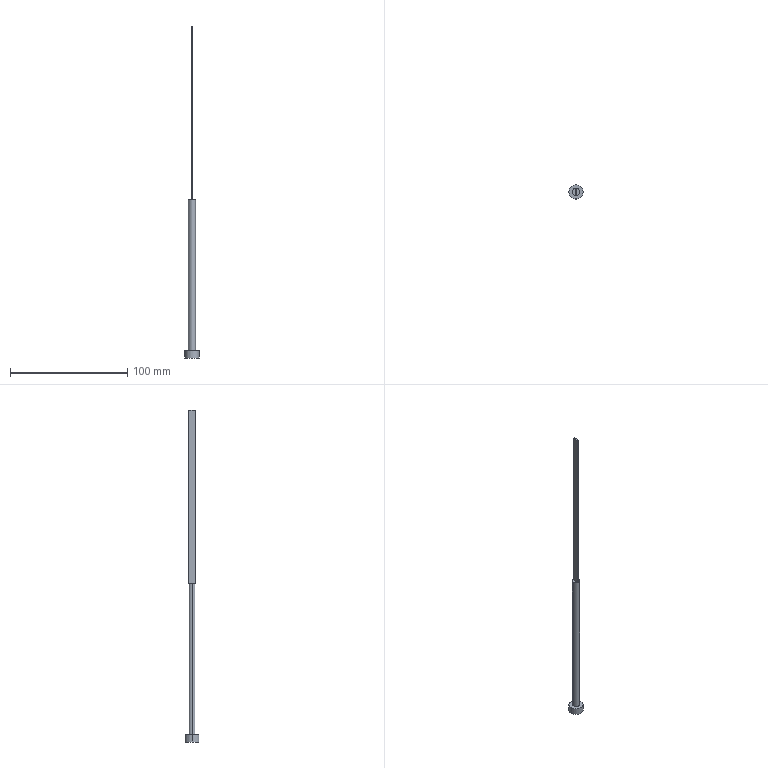Part | Creo | 1 solid | 12 faces | box 12 x 12 x 282.599 mm | volume 5300 mm3 | plane 8 | cylinder 4 | commonest cylinder face diameters 6 x2 12 x2
STEP:
#1=CARTESIAN_POINT('',(-105.609,-1.1,22.099));
#2=VERTEX_POINT('',#1);
#3=CARTESIAN_POINT('',(-105.609,-1.1,-125.5));
#4=VERTEX_POINT('',#3);
#5=CARTESIAN_POINT('',(-105.609,-1.1,22.099));
#6=DIRECTION('',(0.,0.,-1.));
#7=VECTOR('',#6,147.599);
#8=LINE('',#5,#7);
#9=EDGE_CURVE('',#2,#4,#8,.T.);
#10=ORIENTED_EDGE('',*,*,#9,.F.);
#11=CARTESIAN_POINT('',(-105.609,-6.6,22.099));
#12=VERTEX_POINT('',#11);
#13=CARTESIAN_POINT('',(-105.609,-1.1,22.099));
#14=DIRECTION('',(0.,-1.,0.));
#15=VECTOR('',#14,5.5);
#16=LINE('',#13,#15);
#17=EDGE_CURVE('',#2,#12,#16,.T.);
#18=ORIENTED_EDGE('',*,*,#17,.T.);
#19=CARTESIAN_POINT('',(-105.609,-6.6,-125.5));
#20=VERTEX_POINT('',#19);
#21=CARTESIAN_POINT('',(-105.609,-6.6,22.099));
#22=DIRECTION('',(0.,0.,-1.));
#23=VECTOR('',#22,147.599);
#24=LINE('',#21,#23);
#25=EDGE_CURVE('',#12,#20,#24,.T.);
#26=ORIENTED_EDGE('',*,*,#25,.T.);
#27=CARTESIAN_POINT('',(-105.609,-6.6,-125.5));
#28=DIRECTION('',(0.,1.,0.));
#29=VECTOR('',#28,5.5);
#30=LINE('',#27,#29);
#31=EDGE_CURVE('',#20,#4,#30,.T.);
#32=ORIENTED_EDGE('',*,*,#31,.T.);
#33=EDGE_LOOP('',(#10,#18,#26,#32));
#34=FACE_OUTER_BOUND('',#33,.F.);
#35=CARTESIAN_POINT('',(-105.609,-6.6,-77.901));
#36=DIRECTION('',(1.,0.,0.));
#37=DIRECTION('',(0.,1.,0.));
#38=AXIS2_PLACEMENT_3D('',#35,#36,#37);
#39=PLANE('',#38);
#40=ADVANCED_FACE('',(#34),#39,.F.);
#41=CARTESIAN_POINT('',(-104.409,-1.1,22.099));
#42=VERTEX_POINT('',#41);
#43=CARTESIAN_POINT('',(-104.409,-1.1,-125.5));
#44=VERTEX_POINT('',#43);
#45=CARTESIAN_POINT('',(-104.409,-1.1,22.099));
#46=DIRECTION('',(0.,0.,-1.));
#47=VECTOR('',#46,147.599);
#48=LINE('',#45,#47);
#49=EDGE_CURVE('',#42,#44,#48,.T.);
#50=ORIENTED_EDGE('',*,*,#49,.F.);
#51=CARTESIAN_POINT('',(-104.409,-1.1,22.099));
#52=DIRECTION('',(-1.,0.,0.));
#53=VECTOR('',#52,1.2);
#54=LINE('',#51,#53);
#55=EDGE_CURVE('',#42,#2,#54,.T.);
#56=ORIENTED_EDGE('',*,*,#55,.T.);
#57=ORIENTED_EDGE('',*,*,#9,.T.);
#58=CARTESIAN_POINT('',(-105.609,-1.1,-125.5));
#59=DIRECTION('',(1.,0.,0.));
#60=VECTOR('',#59,1.2);
#61=LINE('',#58,#60);
#62=EDGE_CURVE('',#4,#44,#61,.T.);
#63=ORIENTED_EDGE('',*,*,#62,.T.);
#64=EDGE_LOOP('',(#50,#56,#57,#63));
#65=FACE_OUTER_BOUND('',#64,.F.);
#66=CARTESIAN_POINT('',(-105.609,-1.1,-77.901));
#67=DIRECTION('',(0.,-1.,0.));
#68=DIRECTION('',(1.,0.,0.));
#69=AXIS2_PLACEMENT_3D('',#66,#67,#68);
#70=PLANE('',#69);
#71=ADVANCED_FACE('',(#65),#70,.F.);
#72=CARTESIAN_POINT('',(-104.409,-6.6,22.099));
#73=VERTEX_POINT('',#72);
#74=CARTESIAN_POINT('',(-104.409,-6.6,-125.5));
#75=VERTEX_POINT('',#74);
#76=CARTESIAN_POINT('',(-104.409,-6.6,22.099));
#77=DIRECTION('',(0.,0.,-1.));
#78=VECTOR('',#77,147.599);
#79=LINE('',#76,#78);
#80=EDGE_CURVE('',#73,#75,#79,.T.);
#81=ORIENTED_EDGE('',*,*,#80,.F.);
#82=CARTESIAN_POINT('',(-104.409,-6.6,22.099));
#83=DIRECTION('',(0.,1.,0.));
#84=VECTOR('',#83,5.5);
#85=LINE('',#82,#84);
#86=EDGE_CURVE('',#73,#42,#85,.T.);
#87=ORIENTED_EDGE('',*,*,#86,.T.);
#88=ORIENTED_EDGE('',*,*,#49,.T.);
#89=CARTESIAN_POINT('',(-104.409,-1.1,-125.5));
#90=DIRECTION('',(0.,-1.,0.));
#91=VECTOR('',#90,5.5);
#92=LINE('',#89,#91);
#93=EDGE_CURVE('',#44,#75,#92,.T.);
#94=ORIENTED_EDGE('',*,*,#93,.T.);
#95=EDGE_LOOP('',(#81,#87,#88,#94));
#96=FACE_OUTER_BOUND('',#95,.F.);
#97=CARTESIAN_POINT('',(-104.409,-1.1,-77.901));
#98=DIRECTION('',(-1.,0.,0.));
#99=DIRECTION('',(0.,-1.,0.));
#100=AXIS2_PLACEMENT_3D('',#97,#98,#99);
#101=PLANE('',#100);
#102=ADVANCED_FACE('',(#96),#101,.F.);
#103=ORIENTED_EDGE('',*,*,#25,.F.);
#104=CARTESIAN_POINT('',(-105.609,-6.6,22.099));
#105=DIRECTION('',(1.,0.,0.));
#106=VECTOR('',#105,1.2);
#107=LINE('',#104,#106);
#108=EDGE_CURVE('',#12,#73,#107,.T.);
#109=ORIENTED_EDGE('',*,*,#108,.T.);
#110=ORIENTED_EDGE('',*,*,#80,.T.);
#111=CARTESIAN_POINT('',(-104.409,-6.6,-125.5));
#112=DIRECTION('',(-1.,0.,0.));
#113=VECTOR('',#112,1.2);
#114=LINE('',#111,#113);
#115=EDGE_CURVE('',#75,#20,#114,.T.);
#116=ORIENTED_EDGE('',*,*,#115,.T.);
#117=EDGE_LOOP('',(#103,#109,#110,#116));
#118=FACE_OUTER_BOUND('',#117,.F.);
#119=CARTESIAN_POINT('',(-104.409,-6.6,-77.901));
#120=DIRECTION('',(0.,1.,0.));
#121=DIRECTION('',(-1.,0.,0.));
#122=AXIS2_PLACEMENT_3D('',#119,#120,#121);
#123=PLANE('',#122);
#124=ADVANCED_FACE('',(#118),#123,.F.);
#125=ORIENTED_EDGE('',*,*,#17,.F.);
#126=ORIENTED_EDGE('',*,*,#55,.F.);
#127=ORIENTED_EDGE('',*,*,#86,.F.);
#128=ORIENTED_EDGE('',*,*,#108,.F.);
#129=EDGE_LOOP('',(#125,#126,#127,#128));
#130=FACE_OUTER_BOUND('',#129,.F.);
#131=CARTESIAN_POINT('',(-0.003698,-18.777,22.099));
#132=DIRECTION('',(0.,0.,1.));
#133=DIRECTION('',(0.,1.,0.));
#134=AXIS2_PLACEMENT_3D('',#131,#132,#133);
#135=PLANE('',#134);
#136=ADVANCED_FACE('',(#130),#135,.T.);
#137=CARTESIAN_POINT('',(-102.009,-3.85,-125.5));
#138=VERTEX_POINT('',#137);
#139=CARTESIAN_POINT('',(-108.009,-3.85,-125.5));
#140=VERTEX_POINT('',#139);
#141=CARTESIAN_POINT('',(-105.009,-3.85,-125.5));
#142=DIRECTION('',(0.,0.,1.));
#143=DIRECTION('',(1.,0.,0.));
#144=AXIS2_PLACEMENT_3D('',#141,#142,#143);
#145=CIRCLE('',#144,3.);
#146=EDGE_CURVE('',#138,#140,#145,.T.);
#147=ORIENTED_EDGE('',*,*,#146,.F.);
#148=CARTESIAN_POINT('',(-105.009,-3.85,-125.5));
#149=DIRECTION('',(0.,0.,1.));
#150=DIRECTION('',(-1.,0.,0.));
#151=AXIS2_PLACEMENT_3D('',#148,#149,#150);
#152=CIRCLE('',#151,3.);
#153=EDGE_CURVE('',#140,#138,#152,.T.);
#154=ORIENTED_EDGE('',*,*,#153,.F.);
#155=EDGE_LOOP('',(#147,#154));
#156=FACE_OUTER_BOUND('',#155,.F.);
#157=ORIENTED_EDGE('',*,*,#31,.F.);
#158=ORIENTED_EDGE('',*,*,#115,.F.);
#159=ORIENTED_EDGE('',*,*,#93,.F.);
#160=ORIENTED_EDGE('',*,*,#62,.F.);
#161=EDGE_LOOP('',(#157,#158,#159,#160));
#162=FACE_BOUND('',#161,.F.);
#163=CARTESIAN_POINT('',(-105.009,-3.85,-125.5));
#164=DIRECTION('',(0.,0.,1.));
#165=DIRECTION('',(1.,0.,0.));
#166=AXIS2_PLACEMENT_3D('',#163,#164,#165);
#167=PLANE('',#166);
#168=ADVANCED_FACE('',(#156,#162),#167,.T.);
#169=CARTESIAN_POINT('',(-108.009,-3.85,-254.5));
#170=VERTEX_POINT('',#169);
#171=CARTESIAN_POINT('',(-102.009,-3.85,-254.5));
#172=VERTEX_POINT('',#171);
#173=CARTESIAN_POINT('',(-105.009,-3.85,-254.5));
#174=DIRECTION('',(0.,0.,-1.));
#175=DIRECTION('',(-1.,0.,0.));
#176=AXIS2_PLACEMENT_3D('',#173,#174,#175);
#177=CIRCLE('',#176,3.);
#178=EDGE_CURVE('',#170,#172,#177,.T.);
#179=ORIENTED_EDGE('',*,*,#178,.T.);
#180=CARTESIAN_POINT('',(-102.009,-3.85,-254.5));
#181=DIRECTION('',(0.,0.,1.));
#182=VECTOR('',#181,129.);
#183=LINE('',#180,#182);
#184=EDGE_CURVE('',#172,#138,#183,.T.);
#185=ORIENTED_EDGE('',*,*,#184,.T.);
#186=ORIENTED_EDGE('',*,*,#146,.T.);
#187=CARTESIAN_POINT('',(-108.009,-3.85,-254.5));
#188=DIRECTION('',(0.,0.,1.));
#189=VECTOR('',#188,129.);
#190=LINE('',#187,#189);
#191=EDGE_CURVE('',#170,#140,#190,.T.);
#192=ORIENTED_EDGE('',*,*,#191,.F.);
#193=EDGE_LOOP('',(#179,#185,#186,#192));
#194=FACE_OUTER_BOUND('',#193,.F.);
#195=CARTESIAN_POINT('',(-105.009,-3.85,-260.5));
#196=DIRECTION('',(0.,0.,1.));
#197=DIRECTION('',(1.,0.,0.));
#198=AXIS2_PLACEMENT_3D('',#195,#196,#197);
#199=CYLINDRICAL_SURFACE('',#198,3.);
#200=ADVANCED_FACE('',(#194),#199,.T.);
#201=CARTESIAN_POINT('',(-99.009,-3.85,-254.5));
#202=VERTEX_POINT('',#201);
#203=CARTESIAN_POINT('',(-111.009,-3.85,-254.5));
#204=VERTEX_POINT('',#203);
#205=CARTESIAN_POINT('',(-105.009,-3.85,-254.5));
#206=DIRECTION('',(0.,0.,1.));
#207=DIRECTION('',(1.,0.,0.));
#208=AXIS2_PLACEMENT_3D('',#205,#206,#207);
#209=CIRCLE('',#208,6.);
#210=EDGE_CURVE('',#202,#204,#209,.T.);
#211=ORIENTED_EDGE('',*,*,#210,.F.);
#212=CARTESIAN_POINT('',(-105.009,-3.85,-254.5));
#213=DIRECTION('',(0.,0.,1.));
#214=DIRECTION('',(-1.,0.,0.));
#215=AXIS2_PLACEMENT_3D('',#212,#213,#214);
#216=CIRCLE('',#215,6.);
#217=EDGE_CURVE('',#204,#202,#216,.T.);
#218=ORIENTED_EDGE('',*,*,#217,.F.);
#219=EDGE_LOOP('',(#211,#218));
#220=FACE_OUTER_BOUND('',#219,.F.);
#221=CARTESIAN_POINT('',(-105.009,-3.85,-254.5));
#222=DIRECTION('',(0.,0.,-1.));
#223=DIRECTION('',(1.,0.,0.));
#224=AXIS2_PLACEMENT_3D('',#221,#222,#223);
#225=CIRCLE('',#224,3.);
#226=EDGE_CURVE('',#172,#170,#225,.T.);
#227=ORIENTED_EDGE('',*,*,#226,.F.);
#228=ORIENTED_EDGE('',*,*,#178,.F.);
#229=EDGE_LOOP('',(#227,#228));
#230=FACE_BOUND('',#229,.F.);
#231=CARTESIAN_POINT('',(-105.009,-3.85,-254.5));
#232=DIRECTION('',(0.,0.,1.));
#233=DIRECTION('',(1.,0.,0.));
#234=AXIS2_PLACEMENT_3D('',#231,#232,#233);
#235=PLANE('',#234);
#236=ADVANCED_FACE('',(#220,#230),#235,.T.);
#237=ORIENTED_EDGE('',*,*,#226,.T.);
#238=ORIENTED_EDGE('',*,*,#191,.T.);
#239=ORIENTED_EDGE('',*,*,#153,.T.);
#240=ORIENTED_EDGE('',*,*,#184,.F.);
#241=EDGE_LOOP('',(#237,#238,#239,#240));
#242=FACE_OUTER_BOUND('',#241,.F.);
#243=CARTESIAN_POINT('',(-105.009,-3.85,-260.5));
#244=DIRECTION('',(0.,0.,1.));
#245=DIRECTION('',(1.,0.,0.));
#246=AXIS2_PLACEMENT_3D('',#243,#244,#245);
#247=CYLINDRICAL_SURFACE('',#246,3.);
#248=ADVANCED_FACE('',(#242),#247,.T.);
#249=ORIENTED_EDGE('',*,*,#210,.T.);
#250=CARTESIAN_POINT('',(-111.009,-3.85,-260.5));
#251=VERTEX_POINT('',#250);
#252=CARTESIAN_POINT('',(-111.009,-3.85,-260.5));
#253=DIRECTION('',(0.,0.,1.));
#254=VECTOR('',#253,6.);
#255=LINE('',#252,#254);
#256=EDGE_CURVE('',#251,#204,#255,.T.);
#257=ORIENTED_EDGE('',*,*,#256,.F.);
#258=CARTESIAN_POINT('',(-99.009,-3.85,-260.5));
#259=VERTEX_POINT('',#258);
#260=CARTESIAN_POINT('',(-105.009,-3.85,-260.5));
#261=DIRECTION('',(0.,0.,-1.));
#262=DIRECTION('',(-1.,0.,0.));
#263=AXIS2_PLACEMENT_3D('',#260,#261,#262);
#264=CIRCLE('',#263,6.);
#265=EDGE_CURVE('',#251,#259,#264,.T.);
#266=ORIENTED_EDGE('',*,*,#265,.T.);
#267=CARTESIAN_POINT('',(-99.009,-3.85,-260.5));
#268=DIRECTION('',(0.,0.,1.));
#269=VECTOR('',#268,6.);
#270=LINE('',#267,#269);
#271=EDGE_CURVE('',#259,#202,#270,.T.);
#272=ORIENTED_EDGE('',*,*,#271,.T.);
#273=EDGE_LOOP('',(#249,#257,#266,#272));
#274=FACE_OUTER_BOUND('',#273,.F.);
#275=CARTESIAN_POINT('',(-105.009,-3.85,-260.5));
#276=DIRECTION('',(0.,0.,1.));
#277=DIRECTION('',(1.,0.,0.));
#278=AXIS2_PLACEMENT_3D('',#275,#276,#277);
#279=CYLINDRICAL_SURFACE('',#278,6.);
#280=ADVANCED_FACE('',(#274),#279,.T.);
#281=ORIENTED_EDGE('',*,*,#217,.T.);
#282=ORIENTED_EDGE('',*,*,#271,.F.);
#283=CARTESIAN_POINT('',(-105.009,-3.85,-260.5));
#284=DIRECTION('',(0.,0.,-1.));
#285=DIRECTION('',(1.,0.,0.));
#286=AXIS2_PLACEMENT_3D('',#283,#284,#285);
#287=CIRCLE('',#286,6.);
#288=EDGE_CURVE('',#259,#251,#287,.T.);
#289=ORIENTED_EDGE('',*,*,#288,.T.);
#290=ORIENTED_EDGE('',*,*,#256,.T.);
#291=EDGE_LOOP('',(#281,#282,#289,#290));
#292=FACE_OUTER_BOUND('',#291,.F.);
#293=CARTESIAN_POINT('',(-105.009,-3.85,-260.5));
#294=DIRECTION('',(0.,0.,1.));
#295=DIRECTION('',(1.,0.,0.));
#296=AXIS2_PLACEMENT_3D('',#293,#294,#295);
#297=CYLINDRICAL_SURFACE('',#296,6.);
#298=ADVANCED_FACE('',(#292),#297,.T.);
#299=ORIENTED_EDGE('',*,*,#288,.F.);
#300=ORIENTED_EDGE('',*,*,#265,.F.);
#301=EDGE_LOOP('',(#299,#300));
#302=FACE_OUTER_BOUND('',#301,.F.);
#303=CARTESIAN_POINT('',(143.614,163.015,-260.5));
#304=DIRECTION('',(0.,0.,-1.));
#305=DIRECTION('',(1.,0.,0.));
#306=AXIS2_PLACEMENT_3D('',#303,#304,#305);
#307=PLANE('',#306);
#308=ADVANCED_FACE('',(#302),#307,.T.);
#309=CLOSED_SHELL('',(#40,#71,#102,#124,#136,#168,#200,#236,#248,#280,#298,#308));
#310=MANIFOLD_SOLID_BREP('',#309);
#311=(LENGTH_UNIT()NAMED_UNIT(*)SI_UNIT(.MILLI.,.METRE.));
#312=UNCERTAINTY_MEASURE_WITH_UNIT(LENGTH_MEASURE(0.02831),#311,'','');
#313=(NAMED_UNIT(*)PLANE_ANGLE_UNIT()SI_UNIT($,.RADIAN.));
#314=PLANE_ANGLE_MEASURE_WITH_UNIT(PLANE_ANGLE_MEASURE(0.01745),#313);
#315=(CONVERSION_BASED_UNIT('DEGREE',#314)NAMED_UNIT(*)PLANE_ANGLE_UNIT());
#316=(NAMED_UNIT(*)SI_UNIT($,.STERADIAN.)SOLID_ANGLE_UNIT());
#317=(GEOMETRIC_REPRESENTATION_CONTEXT(3)GLOBAL_UNCERTAINTY_ASSIGNED_CONTEXT((#312))GLOBAL_UNIT_ASSIGNED_CONTEXT((#311,#315,#316))REPRESENTATION_CONTEXT('',''));
#318=ADVANCED_BREP_SHAPE_REPRESENTATION('',(#310),#317);